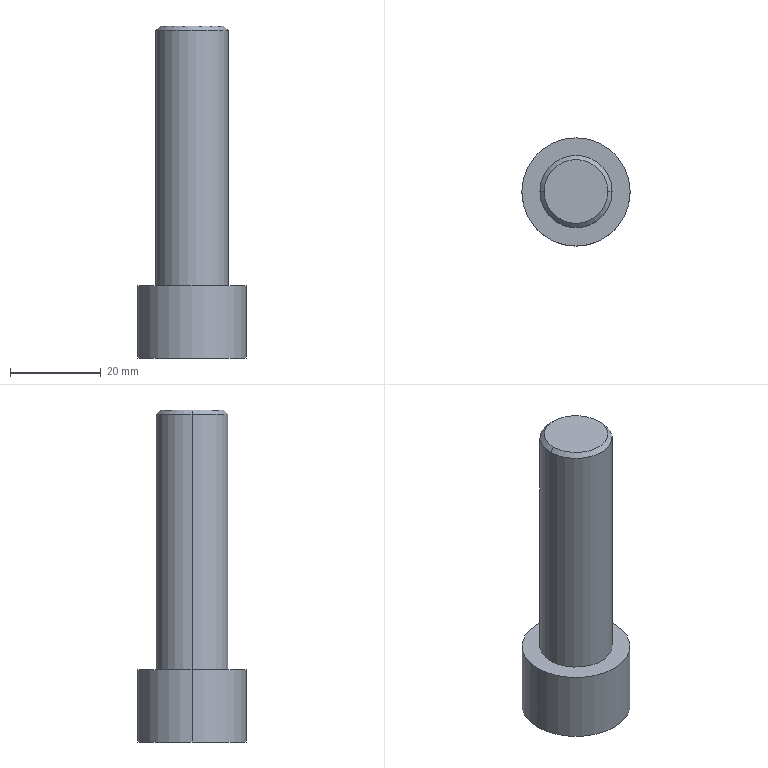Part | STEP file | 4-20.sldasm-Part-320 | 1 solid | 16 faces | box 23.812 x 23.813 x 73.025 mm | volume 16897 mm3 | plane 10 | cylinder 4 | cone 2 | commonest cylinder face diameters 15.875 x2 23.813 x2
STEP:
#1=CARTESIAN_POINT('',(192.,0.,-106.726));
#2=VERTEX_POINT('',#1);
#3=CARTESIAN_POINT('',(178.,0.,-106.726));
#4=VERTEX_POINT('',#3);
#5=CARTESIAN_POINT('',(185.,0.,-106.726));
#6=DIRECTION('',(0.,0.,1.));
#7=DIRECTION('',(-1.,0.,0.));
#8=AXIS2_PLACEMENT_3D('',#5,#6,#7);
#9=CIRCLE('',#8,7.);
#10=EDGE_CURVE('',#2,#4,#9,.T.);
#11=ORIENTED_EDGE('',*,*,#10,.F.);
#12=CARTESIAN_POINT('',(192.937,0.,-107.663));
#13=VERTEX_POINT('',#12);
#14=CARTESIAN_POINT('',(192.937,0.,-107.663));
#15=DIRECTION('',(0.7071,0.,-0.7071));
#16=VECTOR('',#15,1000.);
#17=LINE('',#14,#16);
#18=EDGE_CURVE('',#2,#13,#17,.T.);
#19=ORIENTED_EDGE('',*,*,#18,.T.);
#20=CARTESIAN_POINT('',(177.062,0.,-107.663));
#21=VERTEX_POINT('',#20);
#22=CARTESIAN_POINT('',(185.,0.,-107.663));
#23=DIRECTION('',(0.,0.,-1.));
#24=DIRECTION('',(-1.,0.,0.));
#25=AXIS2_PLACEMENT_3D('',#22,#23,#24);
#26=CIRCLE('',#25,7.937);
#27=EDGE_CURVE('',#21,#13,#26,.T.);
#28=ORIENTED_EDGE('',*,*,#27,.F.);
#29=CARTESIAN_POINT('',(177.062,0.,-107.663));
#30=DIRECTION('',(-0.7071,0.,-0.7071));
#31=VECTOR('',#30,1000.);
#32=LINE('',#29,#31);
#33=EDGE_CURVE('',#4,#21,#32,.T.);
#34=ORIENTED_EDGE('',*,*,#33,.F.);
#35=EDGE_LOOP('',(#11,#19,#28,#34));
#36=FACE_OUTER_BOUND('',#35,.T.);
#37=CARTESIAN_POINT('',(185.,0.,-107.663));
#38=DIRECTION('',(0.,0.,-1.));
#39=DIRECTION('',(-1.,0.,0.));
#40=AXIS2_PLACEMENT_3D('',#37,#38,#39);
#41=CONICAL_SURFACE('',#40,7.937,0.7854);
#42=ADVANCED_FACE('',(#36),#41,.T.);
#43=CARTESIAN_POINT('',(173.094,0.,-163.876));
#44=VERTEX_POINT('',#43);
#45=CARTESIAN_POINT('',(196.906,0.,-163.876));
#46=VERTEX_POINT('',#45);
#47=CARTESIAN_POINT('',(185.,0.,-163.876));
#48=DIRECTION('',(0.,0.,-1.));
#49=DIRECTION('',(-1.,0.,0.));
#50=AXIS2_PLACEMENT_3D('',#47,#48,#49);
#51=CIRCLE('',#50,11.906);
#52=EDGE_CURVE('',#44,#46,#51,.T.);
#53=ORIENTED_EDGE('',*,*,#52,.T.);
#54=CARTESIAN_POINT('',(196.906,0.,-179.751));
#55=VERTEX_POINT('',#54);
#56=CARTESIAN_POINT('',(196.906,0.,-163.876));
#57=DIRECTION('',(0.,0.,-1.));
#58=VECTOR('',#57,1000.);
#59=LINE('',#56,#58);
#60=EDGE_CURVE('',#46,#55,#59,.T.);
#61=ORIENTED_EDGE('',*,*,#60,.T.);
#62=CARTESIAN_POINT('',(173.094,0.,-179.751));
#63=VERTEX_POINT('',#62);
#64=CARTESIAN_POINT('',(185.,0.,-179.751));
#65=DIRECTION('',(0.,0.,-1.));
#66=DIRECTION('',(-1.,0.,0.));
#67=AXIS2_PLACEMENT_3D('',#64,#65,#66);
#68=CIRCLE('',#67,11.906);
#69=EDGE_CURVE('',#63,#55,#68,.T.);
#70=ORIENTED_EDGE('',*,*,#69,.F.);
#71=CARTESIAN_POINT('',(173.094,0.,-163.876));
#72=DIRECTION('',(0.,0.,-1.));
#73=VECTOR('',#72,1000.);
#74=LINE('',#71,#73);
#75=EDGE_CURVE('',#44,#63,#74,.T.);
#76=ORIENTED_EDGE('',*,*,#75,.F.);
#77=EDGE_LOOP('',(#53,#61,#70,#76));
#78=FACE_OUTER_BOUND('',#77,.T.);
#79=CARTESIAN_POINT('',(185.,0.,-163.876));
#80=DIRECTION('',(0.,0.,-1.));
#81=DIRECTION('',(-1.,0.,0.));
#82=AXIS2_PLACEMENT_3D('',#79,#80,#81);
#83=CYLINDRICAL_SURFACE('',#82,11.906);
#84=ADVANCED_FACE('',(#78),#83,.T.);
#85=CARTESIAN_POINT('',(177.062,0.,-163.876));
#86=VERTEX_POINT('',#85);
#87=CARTESIAN_POINT('',(192.937,0.,-163.876));
#88=VERTEX_POINT('',#87);
#89=CARTESIAN_POINT('',(185.,0.,-163.876));
#90=DIRECTION('',(0.,0.,-1.));
#91=DIRECTION('',(-1.,0.,0.));
#92=AXIS2_PLACEMENT_3D('',#89,#90,#91);
#93=CIRCLE('',#92,7.937);
#94=EDGE_CURVE('',#86,#88,#93,.T.);
#95=ORIENTED_EDGE('',*,*,#94,.F.);
#96=CARTESIAN_POINT('',(177.062,0.,-163.876));
#97=DIRECTION('',(0.,0.,1.));
#98=VECTOR('',#97,1000.);
#99=LINE('',#96,#98);
#100=EDGE_CURVE('',#86,#21,#99,.T.);
#101=ORIENTED_EDGE('',*,*,#100,.T.);
#102=ORIENTED_EDGE('',*,*,#27,.T.);
#103=CARTESIAN_POINT('',(192.937,0.,-163.876));
#104=DIRECTION('',(0.,0.,1.));
#105=VECTOR('',#104,1000.);
#106=LINE('',#103,#105);
#107=EDGE_CURVE('',#88,#13,#106,.T.);
#108=ORIENTED_EDGE('',*,*,#107,.F.);
#109=EDGE_LOOP('',(#95,#101,#102,#108));
#110=FACE_OUTER_BOUND('',#109,.T.);
#111=CARTESIAN_POINT('',(185.,0.,-163.876));
#112=DIRECTION('',(0.,0.,1.));
#113=DIRECTION('',(1.,0.,0.));
#114=AXIS2_PLACEMENT_3D('',#111,#112,#113);
#115=CYLINDRICAL_SURFACE('',#114,7.937);
#116=ADVANCED_FACE('',(#110),#115,.T.);
#117=ORIENTED_EDGE('',*,*,#100,.F.);
#118=CARTESIAN_POINT('',(185.,0.,-163.876));
#119=DIRECTION('',(0.,0.,-1.));
#120=DIRECTION('',(-1.,0.,0.));
#121=AXIS2_PLACEMENT_3D('',#118,#119,#120);
#122=CIRCLE('',#121,7.937);
#123=EDGE_CURVE('',#88,#86,#122,.T.);
#124=ORIENTED_EDGE('',*,*,#123,.F.);
#125=ORIENTED_EDGE('',*,*,#107,.T.);
#126=CARTESIAN_POINT('',(185.,0.,-107.663));
#127=DIRECTION('',(0.,0.,-1.));
#128=DIRECTION('',(-1.,0.,0.));
#129=AXIS2_PLACEMENT_3D('',#126,#127,#128);
#130=CIRCLE('',#129,7.937);
#131=EDGE_CURVE('',#13,#21,#130,.T.);
#132=ORIENTED_EDGE('',*,*,#131,.T.);
#133=EDGE_LOOP('',(#117,#124,#125,#132));
#134=FACE_OUTER_BOUND('',#133,.T.);
#135=CARTESIAN_POINT('',(185.,0.,-163.876));
#136=DIRECTION('',(0.,0.,1.));
#137=DIRECTION('',(1.,0.,0.));
#138=AXIS2_PLACEMENT_3D('',#135,#136,#137);
#139=CYLINDRICAL_SURFACE('',#138,7.937);
#140=ADVANCED_FACE('',(#134),#139,.T.);
#141=CARTESIAN_POINT('',(185.,0.,-106.726));
#142=DIRECTION('',(0.,0.,1.));
#143=DIRECTION('',(-1.,0.,0.));
#144=AXIS2_PLACEMENT_3D('',#141,#142,#143);
#145=CIRCLE('',#144,7.);
#146=EDGE_CURVE('',#4,#2,#145,.T.);
#147=ORIENTED_EDGE('',*,*,#146,.T.);
#148=ORIENTED_EDGE('',*,*,#10,.T.);
#149=EDGE_LOOP('',(#147,#148));
#150=FACE_OUTER_BOUND('',#149,.T.);
#151=CARTESIAN_POINT('',(185.,0.,-106.726));
#152=DIRECTION('',(0.,0.,-1.));
#153=DIRECTION('',(-1.,0.,0.));
#154=AXIS2_PLACEMENT_3D('',#151,#152,#153);
#155=PLANE('',#154);
#156=ADVANCED_FACE('',(#150),#155,.F.);
#157=ORIENTED_EDGE('',*,*,#52,.F.);
#158=CARTESIAN_POINT('',(185.,0.,-163.876));
#159=DIRECTION('',(0.,0.,-1.));
#160=DIRECTION('',(-1.,0.,0.));
#161=AXIS2_PLACEMENT_3D('',#158,#159,#160);
#162=CIRCLE('',#161,11.906);
#163=EDGE_CURVE('',#46,#44,#162,.T.);
#164=ORIENTED_EDGE('',*,*,#163,.F.);
#165=EDGE_LOOP('',(#157,#164));
#166=FACE_OUTER_BOUND('',#165,.T.);
#167=ORIENTED_EDGE('',*,*,#123,.T.);
#168=ORIENTED_EDGE('',*,*,#94,.T.);
#169=EDGE_LOOP('',(#167,#168));
#170=FACE_BOUND('',#169,.T.);
#171=CARTESIAN_POINT('',(185.,0.,-163.876));
#172=DIRECTION('',(0.,0.,1.));
#173=DIRECTION('',(1.,0.,0.));
#174=AXIS2_PLACEMENT_3D('',#171,#172,#173);
#175=PLANE('',#174);
#176=ADVANCED_FACE('',(#166,#170),#175,.T.);
#177=CARTESIAN_POINT('',(188.666,-6.35,-179.751));
#178=VERTEX_POINT('',#177);
#179=CARTESIAN_POINT('',(181.334,-6.35,-179.751));
#180=VERTEX_POINT('',#179);
#181=CARTESIAN_POINT('',(188.666,-6.35,-179.751));
#182=DIRECTION('',(-1.,0.,0.));
#183=VECTOR('',#182,1000.);
#184=LINE('',#181,#183);
#185=EDGE_CURVE('',#178,#180,#184,.T.);
#186=ORIENTED_EDGE('',*,*,#185,.F.);
#187=CARTESIAN_POINT('',(192.332,0.,-179.751));
#188=VERTEX_POINT('',#187);
#189=CARTESIAN_POINT('',(192.332,0.,-179.751));
#190=DIRECTION('',(-0.5,-0.866,0.));
#191=VECTOR('',#190,1000.);
#192=LINE('',#189,#191);
#193=EDGE_CURVE('',#188,#178,#192,.T.);
#194=ORIENTED_EDGE('',*,*,#193,.F.);
#195=CARTESIAN_POINT('',(188.666,6.35,-179.751));
#196=VERTEX_POINT('',#195);
#197=CARTESIAN_POINT('',(188.666,6.35,-179.751));
#198=DIRECTION('',(0.5,-0.866,0.));
#199=VECTOR('',#198,1000.);
#200=LINE('',#197,#199);
#201=EDGE_CURVE('',#196,#188,#200,.T.);
#202=ORIENTED_EDGE('',*,*,#201,.F.);
#203=CARTESIAN_POINT('',(181.334,6.35,-179.751));
#204=VERTEX_POINT('',#203);
#205=CARTESIAN_POINT('',(181.334,6.35,-179.751));
#206=DIRECTION('',(1.,0.,0.));
#207=VECTOR('',#206,1000.);
#208=LINE('',#205,#207);
#209=EDGE_CURVE('',#204,#196,#208,.T.);
#210=ORIENTED_EDGE('',*,*,#209,.F.);
#211=CARTESIAN_POINT('',(177.668,0.,-179.751));
#212=VERTEX_POINT('',#211);
#213=CARTESIAN_POINT('',(177.668,0.,-179.751));
#214=DIRECTION('',(0.5,0.866,0.));
#215=VECTOR('',#214,1000.);
#216=LINE('',#213,#215);
#217=EDGE_CURVE('',#212,#204,#216,.T.);
#218=ORIENTED_EDGE('',*,*,#217,.F.);
#219=CARTESIAN_POINT('',(181.334,-6.35,-179.751));
#220=DIRECTION('',(-0.5,0.866,0.));
#221=VECTOR('',#220,1000.);
#222=LINE('',#219,#221);
#223=EDGE_CURVE('',#180,#212,#222,.T.);
#224=ORIENTED_EDGE('',*,*,#223,.F.);
#225=EDGE_LOOP('',(#186,#194,#202,#210,#218,#224));
#226=FACE_BOUND('',#225,.T.);
#227=ORIENTED_EDGE('',*,*,#69,.T.);
#228=CARTESIAN_POINT('',(185.,0.,-179.751));
#229=DIRECTION('',(0.,0.,-1.));
#230=DIRECTION('',(-1.,0.,0.));
#231=AXIS2_PLACEMENT_3D('',#228,#229,#230);
#232=CIRCLE('',#231,11.906);
#233=EDGE_CURVE('',#55,#63,#232,.T.);
#234=ORIENTED_EDGE('',*,*,#233,.T.);
#235=EDGE_LOOP('',(#227,#234));
#236=FACE_OUTER_BOUND('',#235,.T.);
#237=CARTESIAN_POINT('',(185.,0.,-179.751));
#238=DIRECTION('',(0.,0.,-1.));
#239=DIRECTION('',(-1.,0.,0.));
#240=AXIS2_PLACEMENT_3D('',#237,#238,#239);
#241=PLANE('',#240);
#242=ADVANCED_FACE('',(#226,#236),#241,.T.);
#243=ORIENTED_EDGE('',*,*,#60,.F.);
#244=ORIENTED_EDGE('',*,*,#163,.T.);
#245=ORIENTED_EDGE('',*,*,#75,.T.);
#246=ORIENTED_EDGE('',*,*,#233,.F.);
#247=EDGE_LOOP('',(#243,#244,#245,#246));
#248=FACE_OUTER_BOUND('',#247,.T.);
#249=CARTESIAN_POINT('',(185.,0.,-163.876));
#250=DIRECTION('',(0.,0.,-1.));
#251=DIRECTION('',(-1.,0.,0.));
#252=AXIS2_PLACEMENT_3D('',#249,#250,#251);
#253=CYLINDRICAL_SURFACE('',#252,11.906);
#254=ADVANCED_FACE('',(#248),#253,.T.);
#255=ORIENTED_EDGE('',*,*,#18,.F.);
#256=ORIENTED_EDGE('',*,*,#146,.F.);
#257=ORIENTED_EDGE('',*,*,#33,.T.);
#258=ORIENTED_EDGE('',*,*,#131,.F.);
#259=EDGE_LOOP('',(#255,#256,#257,#258));
#260=FACE_OUTER_BOUND('',#259,.T.);
#261=CARTESIAN_POINT('',(185.,0.,-107.663));
#262=DIRECTION('',(0.,0.,-1.));
#263=DIRECTION('',(-1.,0.,0.));
#264=AXIS2_PLACEMENT_3D('',#261,#262,#263);
#265=CONICAL_SURFACE('',#264,7.937,0.7854);
#266=ADVANCED_FACE('',(#260),#265,.T.);
#267=ORIENTED_EDGE('',*,*,#185,.T.);
#268=CARTESIAN_POINT('',(181.334,-6.35,-169.273));
#269=VERTEX_POINT('',#268);
#270=CARTESIAN_POINT('',(181.334,-6.35,-169.273));
#271=DIRECTION('',(0.,0.,-1.));
#272=VECTOR('',#271,1000.);
#273=LINE('',#270,#272);
#274=EDGE_CURVE('',#269,#180,#273,.T.);
#275=ORIENTED_EDGE('',*,*,#274,.F.);
#276=CARTESIAN_POINT('',(188.666,-6.35,-169.273));
#277=VERTEX_POINT('',#276);
#278=CARTESIAN_POINT('',(188.666,-6.35,-169.273));
#279=DIRECTION('',(-1.,0.,0.));
#280=VECTOR('',#279,1000.);
#281=LINE('',#278,#280);
#282=EDGE_CURVE('',#277,#269,#281,.T.);
#283=ORIENTED_EDGE('',*,*,#282,.F.);
#284=CARTESIAN_POINT('',(188.666,-6.35,-169.273));
#285=DIRECTION('',(0.,0.,-1.));
#286=VECTOR('',#285,1000.);
#287=LINE('',#284,#286);
#288=EDGE_CURVE('',#277,#178,#287,.T.);
#289=ORIENTED_EDGE('',*,*,#288,.T.);
#290=EDGE_LOOP('',(#267,#275,#283,#289));
#291=FACE_OUTER_BOUND('',#290,.T.);
#292=CARTESIAN_POINT('',(188.666,-6.35,-169.273));
#293=DIRECTION('',(0.,-1.,0.));
#294=DIRECTION('',(0.,0.,1.));
#295=AXIS2_PLACEMENT_3D('',#292,#293,#294);
#296=PLANE('',#295);
#297=ADVANCED_FACE('',(#291),#296,.F.);
#298=ORIENTED_EDGE('',*,*,#223,.T.);
#299=CARTESIAN_POINT('',(177.668,0.,-169.273));
#300=VERTEX_POINT('',#299);
#301=CARTESIAN_POINT('',(177.668,0.,-169.273));
#302=DIRECTION('',(0.,0.,-1.));
#303=VECTOR('',#302,1000.);
#304=LINE('',#301,#303);
#305=EDGE_CURVE('',#300,#212,#304,.T.);
#306=ORIENTED_EDGE('',*,*,#305,.F.);
#307=CARTESIAN_POINT('',(181.334,-6.35,-169.273));
#308=DIRECTION('',(-0.5,0.866,0.));
#309=VECTOR('',#308,1000.);
#310=LINE('',#307,#309);
#311=EDGE_CURVE('',#269,#300,#310,.T.);
#312=ORIENTED_EDGE('',*,*,#311,.F.);
#313=ORIENTED_EDGE('',*,*,#274,.T.);
#314=EDGE_LOOP('',(#298,#306,#312,#313));
#315=FACE_OUTER_BOUND('',#314,.T.);
#316=CARTESIAN_POINT('',(181.334,-6.35,-169.273));
#317=DIRECTION('',(-0.866,-0.5,0.));
#318=DIRECTION('',(-0.5,0.866,0.));
#319=AXIS2_PLACEMENT_3D('',#316,#317,#318);
#320=PLANE('',#319);
#321=ADVANCED_FACE('',(#315),#320,.F.);
#322=ORIENTED_EDGE('',*,*,#217,.T.);
#323=CARTESIAN_POINT('',(181.334,6.35,-169.273));
#324=VERTEX_POINT('',#323);
#325=CARTESIAN_POINT('',(181.334,6.35,-169.273));
#326=DIRECTION('',(0.,0.,-1.));
#327=VECTOR('',#326,1000.);
#328=LINE('',#325,#327);
#329=EDGE_CURVE('',#324,#204,#328,.T.);
#330=ORIENTED_EDGE('',*,*,#329,.F.);
#331=CARTESIAN_POINT('',(177.668,0.,-169.273));
#332=DIRECTION('',(0.5,0.866,0.));
#333=VECTOR('',#332,1000.);
#334=LINE('',#331,#333);
#335=EDGE_CURVE('',#300,#324,#334,.T.);
#336=ORIENTED_EDGE('',*,*,#335,.F.);
#337=ORIENTED_EDGE('',*,*,#305,.T.);
#338=EDGE_LOOP('',(#322,#330,#336,#337));
#339=FACE_OUTER_BOUND('',#338,.T.);
#340=CARTESIAN_POINT('',(177.668,0.,-169.273));
#341=DIRECTION('',(-0.866,0.5,0.));
#342=DIRECTION('',(0.5,0.866,0.));
#343=AXIS2_PLACEMENT_3D('',#340,#341,#342);
#344=PLANE('',#343);
#345=ADVANCED_FACE('',(#339),#344,.F.);
#346=ORIENTED_EDGE('',*,*,#209,.T.);
#347=CARTESIAN_POINT('',(188.666,6.35,-169.273));
#348=VERTEX_POINT('',#347);
#349=CARTESIAN_POINT('',(188.666,6.35,-169.273));
#350=DIRECTION('',(0.,0.,-1.));
#351=VECTOR('',#350,1000.);
#352=LINE('',#349,#351);
#353=EDGE_CURVE('',#348,#196,#352,.T.);
#354=ORIENTED_EDGE('',*,*,#353,.F.);
#355=CARTESIAN_POINT('',(181.334,6.35,-169.273));
#356=DIRECTION('',(1.,0.,0.));
#357=VECTOR('',#356,1000.);
#358=LINE('',#355,#357);
#359=EDGE_CURVE('',#324,#348,#358,.T.);
#360=ORIENTED_EDGE('',*,*,#359,.F.);
#361=ORIENTED_EDGE('',*,*,#329,.T.);
#362=EDGE_LOOP('',(#346,#354,#360,#361));
#363=FACE_OUTER_BOUND('',#362,.T.);
#364=CARTESIAN_POINT('',(181.334,6.35,-169.273));
#365=DIRECTION('',(0.,1.,0.));
#366=DIRECTION('',(0.,0.,-1.));
#367=AXIS2_PLACEMENT_3D('',#364,#365,#366);
#368=PLANE('',#367);
#369=ADVANCED_FACE('',(#363),#368,.F.);
#370=ORIENTED_EDGE('',*,*,#201,.T.);
#371=CARTESIAN_POINT('',(192.332,0.,-169.273));
#372=VERTEX_POINT('',#371);
#373=CARTESIAN_POINT('',(192.332,0.,-169.273));
#374=DIRECTION('',(0.,0.,-1.));
#375=VECTOR('',#374,1000.);
#376=LINE('',#373,#375);
#377=EDGE_CURVE('',#372,#188,#376,.T.);
#378=ORIENTED_EDGE('',*,*,#377,.F.);
#379=CARTESIAN_POINT('',(188.666,6.35,-169.273));
#380=DIRECTION('',(0.5,-0.866,0.));
#381=VECTOR('',#380,1000.);
#382=LINE('',#379,#381);
#383=EDGE_CURVE('',#348,#372,#382,.T.);
#384=ORIENTED_EDGE('',*,*,#383,.F.);
#385=ORIENTED_EDGE('',*,*,#353,.T.);
#386=EDGE_LOOP('',(#370,#378,#384,#385));
#387=FACE_OUTER_BOUND('',#386,.T.);
#388=CARTESIAN_POINT('',(188.666,6.35,-169.273));
#389=DIRECTION('',(0.866,0.5,0.));
#390=DIRECTION('',(0.5,-0.866,0.));
#391=AXIS2_PLACEMENT_3D('',#388,#389,#390);
#392=PLANE('',#391);
#393=ADVANCED_FACE('',(#387),#392,.F.);
#394=ORIENTED_EDGE('',*,*,#193,.T.);
#395=ORIENTED_EDGE('',*,*,#288,.F.);
#396=CARTESIAN_POINT('',(192.332,0.,-169.273));
#397=DIRECTION('',(-0.5,-0.866,0.));
#398=VECTOR('',#397,1000.);
#399=LINE('',#396,#398);
#400=EDGE_CURVE('',#372,#277,#399,.T.);
#401=ORIENTED_EDGE('',*,*,#400,.F.);
#402=ORIENTED_EDGE('',*,*,#377,.T.);
#403=EDGE_LOOP('',(#394,#395,#401,#402));
#404=FACE_OUTER_BOUND('',#403,.T.);
#405=CARTESIAN_POINT('',(192.332,0.,-169.273));
#406=DIRECTION('',(0.866,-0.5,0.));
#407=DIRECTION('',(-0.5,-0.866,0.));
#408=AXIS2_PLACEMENT_3D('',#405,#406,#407);
#409=PLANE('',#408);
#410=ADVANCED_FACE('',(#404),#409,.F.);
#411=ORIENTED_EDGE('',*,*,#282,.T.);
#412=ORIENTED_EDGE('',*,*,#311,.T.);
#413=ORIENTED_EDGE('',*,*,#335,.T.);
#414=ORIENTED_EDGE('',*,*,#359,.T.);
#415=ORIENTED_EDGE('',*,*,#383,.T.);
#416=ORIENTED_EDGE('',*,*,#400,.T.);
#417=EDGE_LOOP('',(#411,#412,#413,#414,#415,#416));
#418=FACE_OUTER_BOUND('',#417,.T.);
#419=CARTESIAN_POINT('',(181.334,-6.35,-169.273));
#420=DIRECTION('',(0.,0.,-1.));
#421=DIRECTION('',(-1.,0.,0.));
#422=AXIS2_PLACEMENT_3D('',#419,#420,#421);
#423=PLANE('',#422);
#424=ADVANCED_FACE('',(#418),#423,.T.);
#425=CLOSED_SHELL('',(#42,#84,#116,#140,#156,#176,#242,#254,#266,#297,#321,#345,#369,#393,#410,#424));
#426=MANIFOLD_SOLID_BREP('',#425);
#427=CARTESIAN_POINT('',(0.,0.,0.));
#428=DIRECTION('',(0.,0.,1.));
#429=DIRECTION('',(1.,0.,0.));
#430=AXIS2_PLACEMENT_3D('',#427,#428,#429);
#431=(LENGTH_UNIT()NAMED_UNIT(*)SI_UNIT(.MILLI.,.METRE.));
#432=UNCERTAINTY_MEASURE_WITH_UNIT(LENGTH_MEASURE(0.00001),#431,'','');
#433=(NAMED_UNIT(*)PLANE_ANGLE_UNIT()SI_UNIT($,.RADIAN.));
#434=(NAMED_UNIT(*)SI_UNIT($,.STERADIAN.)SOLID_ANGLE_UNIT());
#435=(GEOMETRIC_REPRESENTATION_CONTEXT(3)GLOBAL_UNCERTAINTY_ASSIGNED_CONTEXT((#432))GLOBAL_UNIT_ASSIGNED_CONTEXT((#431,#433,#434))REPRESENTATION_CONTEXT('',''));
#436=ADVANCED_BREP_SHAPE_REPRESENTATION('',(#426,#430),#435);